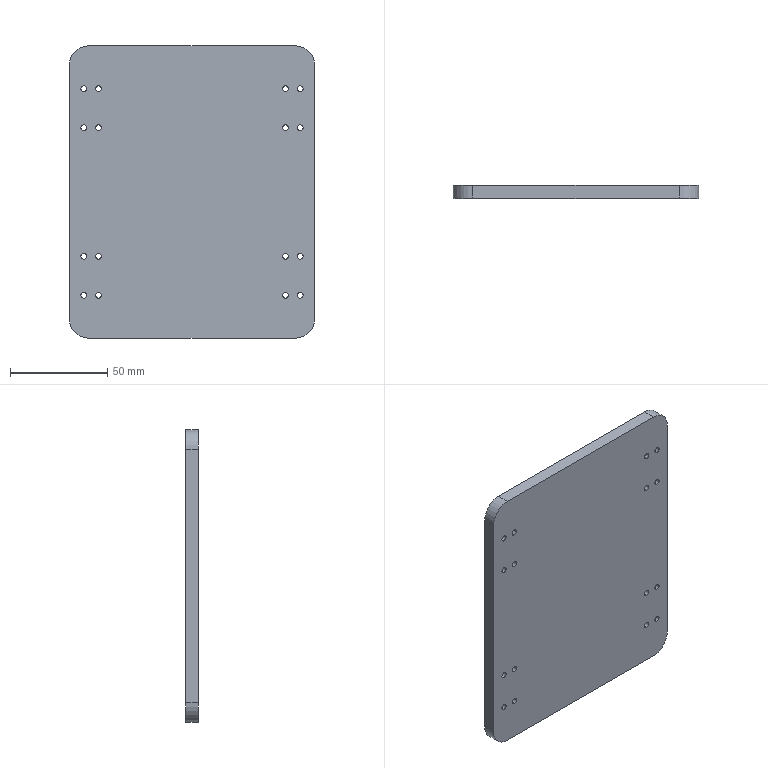Part | SolidWorks | features MirrorPattern 2, Extrusion 1, Fillet 1, ICE 1 | 1 solid | 42 faces | box 126 x 6.5 x 150 mm | volume 121557 mm3 | cylinder 36 | plane 6 | commonest cylinder face diameters 3 x32 20 x4
STEP:
#1=CARTESIAN_POINT('',(55.5,0.,54.5));
#2=VERTEX_POINT('',#1);
#3=CARTESIAN_POINT('',(55.5,0.,51.5));
#4=VERTEX_POINT('',#3);
#5=CARTESIAN_POINT('',(55.5,0.,53.));
#6=DIRECTION('',(0.,-1.,0.));
#7=DIRECTION('',(0.,0.,-1.));
#8=AXIS2_PLACEMENT_3D('',#5,#6,#7);
#9=CIRCLE('',#8,1.5);
#10=EDGE_CURVE('',#2,#4,#9,.T.);
#11=ORIENTED_EDGE('',*,*,#10,.T.);
#12=CARTESIAN_POINT('',(55.5,6.5,51.5));
#13=VERTEX_POINT('',#12);
#14=CARTESIAN_POINT('',(55.5,-3.5,51.5));
#15=DIRECTION('',(0.,1.,0.));
#16=VECTOR('',#15,1000.);
#17=LINE('',#14,#16);
#18=EDGE_CURVE('',#4,#13,#17,.T.);
#19=ORIENTED_EDGE('',*,*,#18,.T.);
#20=CARTESIAN_POINT('',(55.5,6.5,54.5));
#21=VERTEX_POINT('',#20);
#22=CARTESIAN_POINT('',(55.5,6.5,53.));
#23=DIRECTION('',(0.,1.,0.));
#24=DIRECTION('',(0.,0.,1.));
#25=AXIS2_PLACEMENT_3D('',#22,#23,#24);
#26=CIRCLE('',#25,1.5);
#27=EDGE_CURVE('',#13,#21,#26,.T.);
#28=ORIENTED_EDGE('',*,*,#27,.T.);
#29=CARTESIAN_POINT('',(55.5,-3.5,54.5));
#30=DIRECTION('',(0.,1.,0.));
#31=VECTOR('',#30,1000.);
#32=LINE('',#29,#31);
#33=EDGE_CURVE('',#2,#21,#32,.T.);
#34=ORIENTED_EDGE('',*,*,#33,.F.);
#35=EDGE_LOOP('',(#11,#19,#28,#34));
#36=FACE_OUTER_BOUND('',#35,.T.);
#37=CARTESIAN_POINT('',(55.5,-3.5,53.));
#38=DIRECTION('',(0.,1.,0.));
#39=DIRECTION('',(0.,0.,1.));
#40=AXIS2_PLACEMENT_3D('',#37,#38,#39);
#41=CYLINDRICAL_SURFACE('',#40,1.5);
#42=ADVANCED_FACE('',(#36),#41,.F.);
#43=CARTESIAN_POINT('',(48.,0.,54.5));
#44=VERTEX_POINT('',#43);
#45=CARTESIAN_POINT('',(48.,0.,51.5));
#46=VERTEX_POINT('',#45);
#47=CARTESIAN_POINT('',(48.,0.,53.));
#48=DIRECTION('',(0.,-1.,0.));
#49=DIRECTION('',(0.,0.,-1.));
#50=AXIS2_PLACEMENT_3D('',#47,#48,#49);
#51=CIRCLE('',#50,1.5);
#52=EDGE_CURVE('',#44,#46,#51,.T.);
#53=ORIENTED_EDGE('',*,*,#52,.T.);
#54=CARTESIAN_POINT('',(48.,6.5,51.5));
#55=VERTEX_POINT('',#54);
#56=CARTESIAN_POINT('',(48.,-3.5,51.5));
#57=DIRECTION('',(0.,1.,0.));
#58=VECTOR('',#57,1000.);
#59=LINE('',#56,#58);
#60=EDGE_CURVE('',#46,#55,#59,.T.);
#61=ORIENTED_EDGE('',*,*,#60,.T.);
#62=CARTESIAN_POINT('',(48.,6.5,54.5));
#63=VERTEX_POINT('',#62);
#64=CARTESIAN_POINT('',(48.,6.5,53.));
#65=DIRECTION('',(0.,1.,0.));
#66=DIRECTION('',(0.,0.,-1.));
#67=AXIS2_PLACEMENT_3D('',#64,#65,#66);
#68=CIRCLE('',#67,1.5);
#69=EDGE_CURVE('',#55,#63,#68,.T.);
#70=ORIENTED_EDGE('',*,*,#69,.T.);
#71=CARTESIAN_POINT('',(48.,-3.5,54.5));
#72=DIRECTION('',(0.,1.,0.));
#73=VECTOR('',#72,1000.);
#74=LINE('',#71,#73);
#75=EDGE_CURVE('',#44,#63,#74,.T.);
#76=ORIENTED_EDGE('',*,*,#75,.F.);
#77=EDGE_LOOP('',(#53,#61,#70,#76));
#78=FACE_OUTER_BOUND('',#77,.T.);
#79=CARTESIAN_POINT('',(48.,-3.5,53.));
#80=DIRECTION('',(0.,1.,0.));
#81=DIRECTION('',(0.,0.,1.));
#82=AXIS2_PLACEMENT_3D('',#79,#80,#81);
#83=CYLINDRICAL_SURFACE('',#82,1.5);
#84=ADVANCED_FACE('',(#78),#83,.F.);
#85=CARTESIAN_POINT('',(48.,0.,34.5));
#86=VERTEX_POINT('',#85);
#87=CARTESIAN_POINT('',(48.,0.,31.5));
#88=VERTEX_POINT('',#87);
#89=CARTESIAN_POINT('',(48.,0.,33.));
#90=DIRECTION('',(0.,-1.,0.));
#91=DIRECTION('',(0.,0.,-1.));
#92=AXIS2_PLACEMENT_3D('',#89,#90,#91);
#93=CIRCLE('',#92,1.5);
#94=EDGE_CURVE('',#86,#88,#93,.T.);
#95=ORIENTED_EDGE('',*,*,#94,.T.);
#96=CARTESIAN_POINT('',(48.,6.5,31.5));
#97=VERTEX_POINT('',#96);
#98=CARTESIAN_POINT('',(48.,-3.5,31.5));
#99=DIRECTION('',(0.,1.,0.));
#100=VECTOR('',#99,1000.);
#101=LINE('',#98,#100);
#102=EDGE_CURVE('',#88,#97,#101,.T.);
#103=ORIENTED_EDGE('',*,*,#102,.T.);
#104=CARTESIAN_POINT('',(48.,6.5,34.5));
#105=VERTEX_POINT('',#104);
#106=CARTESIAN_POINT('',(48.,6.5,33.));
#107=DIRECTION('',(0.,1.,0.));
#108=DIRECTION('',(0.,0.,1.));
#109=AXIS2_PLACEMENT_3D('',#106,#107,#108);
#110=CIRCLE('',#109,1.5);
#111=EDGE_CURVE('',#97,#105,#110,.T.);
#112=ORIENTED_EDGE('',*,*,#111,.T.);
#113=CARTESIAN_POINT('',(48.,-3.5,34.5));
#114=DIRECTION('',(0.,1.,0.));
#115=VECTOR('',#114,1000.);
#116=LINE('',#113,#115);
#117=EDGE_CURVE('',#86,#105,#116,.T.);
#118=ORIENTED_EDGE('',*,*,#117,.F.);
#119=EDGE_LOOP('',(#95,#103,#112,#118));
#120=FACE_OUTER_BOUND('',#119,.T.);
#121=CARTESIAN_POINT('',(48.,-3.5,33.));
#122=DIRECTION('',(0.,1.,0.));
#123=DIRECTION('',(0.,0.,1.));
#124=AXIS2_PLACEMENT_3D('',#121,#122,#123);
#125=CYLINDRICAL_SURFACE('',#124,1.5);
#126=ADVANCED_FACE('',(#120),#125,.F.);
#127=CARTESIAN_POINT('',(55.5,0.,34.5));
#128=VERTEX_POINT('',#127);
#129=CARTESIAN_POINT('',(55.5,0.,31.5));
#130=VERTEX_POINT('',#129);
#131=CARTESIAN_POINT('',(55.5,0.,33.));
#132=DIRECTION('',(0.,-1.,0.));
#133=DIRECTION('',(0.,0.,-1.));
#134=AXIS2_PLACEMENT_3D('',#131,#132,#133);
#135=CIRCLE('',#134,1.5);
#136=EDGE_CURVE('',#128,#130,#135,.T.);
#137=ORIENTED_EDGE('',*,*,#136,.T.);
#138=CARTESIAN_POINT('',(55.5,6.5,31.5));
#139=VERTEX_POINT('',#138);
#140=CARTESIAN_POINT('',(55.5,-3.5,31.5));
#141=DIRECTION('',(0.,1.,0.));
#142=VECTOR('',#141,1000.);
#143=LINE('',#140,#142);
#144=EDGE_CURVE('',#130,#139,#143,.T.);
#145=ORIENTED_EDGE('',*,*,#144,.T.);
#146=CARTESIAN_POINT('',(55.5,6.5,34.5));
#147=VERTEX_POINT('',#146);
#148=CARTESIAN_POINT('',(55.5,6.5,33.));
#149=DIRECTION('',(0.,1.,0.));
#150=DIRECTION('',(0.,0.,-1.));
#151=AXIS2_PLACEMENT_3D('',#148,#149,#150);
#152=CIRCLE('',#151,1.5);
#153=EDGE_CURVE('',#139,#147,#152,.T.);
#154=ORIENTED_EDGE('',*,*,#153,.T.);
#155=CARTESIAN_POINT('',(55.5,-3.5,34.5));
#156=DIRECTION('',(0.,1.,0.));
#157=VECTOR('',#156,1000.);
#158=LINE('',#155,#157);
#159=EDGE_CURVE('',#128,#147,#158,.T.);
#160=ORIENTED_EDGE('',*,*,#159,.F.);
#161=EDGE_LOOP('',(#137,#145,#154,#160));
#162=FACE_OUTER_BOUND('',#161,.T.);
#163=CARTESIAN_POINT('',(55.5,-3.5,33.));
#164=DIRECTION('',(0.,1.,0.));
#165=DIRECTION('',(0.,0.,1.));
#166=AXIS2_PLACEMENT_3D('',#163,#164,#165);
#167=CYLINDRICAL_SURFACE('',#166,1.5);
#168=ADVANCED_FACE('',(#162),#167,.F.);
#169=CARTESIAN_POINT('',(-55.5,0.,51.5));
#170=VERTEX_POINT('',#169);
#171=CARTESIAN_POINT('',(-55.5,0.,54.5));
#172=VERTEX_POINT('',#171);
#173=CARTESIAN_POINT('',(-55.5,0.,53.));
#174=DIRECTION('',(0.,1.,0.));
#175=DIRECTION('',(0.,0.,-1.));
#176=AXIS2_PLACEMENT_3D('',#173,#174,#175);
#177=CIRCLE('',#176,1.5);
#178=EDGE_CURVE('',#170,#172,#177,.T.);
#179=ORIENTED_EDGE('',*,*,#178,.F.);
#180=CARTESIAN_POINT('',(-55.5,6.5,51.5));
#181=VERTEX_POINT('',#180);
#182=CARTESIAN_POINT('',(-55.5,-3.5,51.5));
#183=DIRECTION('',(0.,1.,0.));
#184=VECTOR('',#183,1000.);
#185=LINE('',#182,#184);
#186=EDGE_CURVE('',#170,#181,#185,.T.);
#187=ORIENTED_EDGE('',*,*,#186,.T.);
#188=CARTESIAN_POINT('',(-55.5,6.5,54.5));
#189=VERTEX_POINT('',#188);
#190=CARTESIAN_POINT('',(-55.5,6.5,53.));
#191=DIRECTION('',(0.,-1.,0.));
#192=DIRECTION('',(0.,0.,1.));
#193=AXIS2_PLACEMENT_3D('',#190,#191,#192);
#194=CIRCLE('',#193,1.5);
#195=EDGE_CURVE('',#189,#181,#194,.T.);
#196=ORIENTED_EDGE('',*,*,#195,.F.);
#197=CARTESIAN_POINT('',(-55.5,-3.5,54.5));
#198=DIRECTION('',(0.,1.,0.));
#199=VECTOR('',#198,1000.);
#200=LINE('',#197,#199);
#201=EDGE_CURVE('',#172,#189,#200,.T.);
#202=ORIENTED_EDGE('',*,*,#201,.F.);
#203=EDGE_LOOP('',(#179,#187,#196,#202));
#204=FACE_OUTER_BOUND('',#203,.T.);
#205=CARTESIAN_POINT('',(-55.5,-3.5,53.));
#206=DIRECTION('',(0.,1.,0.));
#207=DIRECTION('',(0.,0.,1.));
#208=AXIS2_PLACEMENT_3D('',#205,#206,#207);
#209=CYLINDRICAL_SURFACE('',#208,1.5);
#210=ADVANCED_FACE('',(#204),#209,.F.);
#211=CARTESIAN_POINT('',(-48.,0.,51.5));
#212=VERTEX_POINT('',#211);
#213=CARTESIAN_POINT('',(-48.,0.,54.5));
#214=VERTEX_POINT('',#213);
#215=CARTESIAN_POINT('',(-48.,0.,53.));
#216=DIRECTION('',(0.,1.,0.));
#217=DIRECTION('',(0.,0.,-1.));
#218=AXIS2_PLACEMENT_3D('',#215,#216,#217);
#219=CIRCLE('',#218,1.5);
#220=EDGE_CURVE('',#212,#214,#219,.T.);
#221=ORIENTED_EDGE('',*,*,#220,.F.);
#222=CARTESIAN_POINT('',(-48.,6.5,51.5));
#223=VERTEX_POINT('',#222);
#224=CARTESIAN_POINT('',(-48.,-3.5,51.5));
#225=DIRECTION('',(0.,1.,0.));
#226=VECTOR('',#225,1000.);
#227=LINE('',#224,#226);
#228=EDGE_CURVE('',#212,#223,#227,.T.);
#229=ORIENTED_EDGE('',*,*,#228,.T.);
#230=CARTESIAN_POINT('',(-48.,6.5,54.5));
#231=VERTEX_POINT('',#230);
#232=CARTESIAN_POINT('',(-48.,6.5,53.));
#233=DIRECTION('',(0.,-1.,0.));
#234=DIRECTION('',(0.,0.,-1.));
#235=AXIS2_PLACEMENT_3D('',#232,#233,#234);
#236=CIRCLE('',#235,1.5);
#237=EDGE_CURVE('',#231,#223,#236,.T.);
#238=ORIENTED_EDGE('',*,*,#237,.F.);
#239=CARTESIAN_POINT('',(-48.,-3.5,54.5));
#240=DIRECTION('',(0.,1.,0.));
#241=VECTOR('',#240,1000.);
#242=LINE('',#239,#241);
#243=EDGE_CURVE('',#214,#231,#242,.T.);
#244=ORIENTED_EDGE('',*,*,#243,.F.);
#245=EDGE_LOOP('',(#221,#229,#238,#244));
#246=FACE_OUTER_BOUND('',#245,.T.);
#247=CARTESIAN_POINT('',(-48.,-3.5,53.));
#248=DIRECTION('',(0.,1.,0.));
#249=DIRECTION('',(0.,0.,1.));
#250=AXIS2_PLACEMENT_3D('',#247,#248,#249);
#251=CYLINDRICAL_SURFACE('',#250,1.5);
#252=ADVANCED_FACE('',(#246),#251,.F.);
#253=CARTESIAN_POINT('',(-48.,0.,31.5));
#254=VERTEX_POINT('',#253);
#255=CARTESIAN_POINT('',(-48.,0.,34.5));
#256=VERTEX_POINT('',#255);
#257=CARTESIAN_POINT('',(-48.,0.,33.));
#258=DIRECTION('',(0.,1.,0.));
#259=DIRECTION('',(0.,0.,-1.));
#260=AXIS2_PLACEMENT_3D('',#257,#258,#259);
#261=CIRCLE('',#260,1.5);
#262=EDGE_CURVE('',#254,#256,#261,.T.);
#263=ORIENTED_EDGE('',*,*,#262,.F.);
#264=CARTESIAN_POINT('',(-48.,6.5,31.5));
#265=VERTEX_POINT('',#264);
#266=CARTESIAN_POINT('',(-48.,-3.5,31.5));
#267=DIRECTION('',(0.,1.,0.));
#268=VECTOR('',#267,1000.);
#269=LINE('',#266,#268);
#270=EDGE_CURVE('',#254,#265,#269,.T.);
#271=ORIENTED_EDGE('',*,*,#270,.T.);
#272=CARTESIAN_POINT('',(-48.,6.5,34.5));
#273=VERTEX_POINT('',#272);
#274=CARTESIAN_POINT('',(-48.,6.5,33.));
#275=DIRECTION('',(0.,-1.,0.));
#276=DIRECTION('',(0.,0.,1.));
#277=AXIS2_PLACEMENT_3D('',#274,#275,#276);
#278=CIRCLE('',#277,1.5);
#279=EDGE_CURVE('',#273,#265,#278,.T.);
#280=ORIENTED_EDGE('',*,*,#279,.F.);
#281=CARTESIAN_POINT('',(-48.,-3.5,34.5));
#282=DIRECTION('',(0.,1.,0.));
#283=VECTOR('',#282,1000.);
#284=LINE('',#281,#283);
#285=EDGE_CURVE('',#256,#273,#284,.T.);
#286=ORIENTED_EDGE('',*,*,#285,.F.);
#287=EDGE_LOOP('',(#263,#271,#280,#286));
#288=FACE_OUTER_BOUND('',#287,.T.);
#289=CARTESIAN_POINT('',(-48.,-3.5,33.));
#290=DIRECTION('',(0.,1.,0.));
#291=DIRECTION('',(0.,0.,1.));
#292=AXIS2_PLACEMENT_3D('',#289,#290,#291);
#293=CYLINDRICAL_SURFACE('',#292,1.5);
#294=ADVANCED_FACE('',(#288),#293,.F.);
#295=CARTESIAN_POINT('',(-55.5,0.,31.5));
#296=VERTEX_POINT('',#295);
#297=CARTESIAN_POINT('',(-55.5,0.,34.5));
#298=VERTEX_POINT('',#297);
#299=CARTESIAN_POINT('',(-55.5,0.,33.));
#300=DIRECTION('',(0.,1.,0.));
#301=DIRECTION('',(0.,0.,-1.));
#302=AXIS2_PLACEMENT_3D('',#299,#300,#301);
#303=CIRCLE('',#302,1.5);
#304=EDGE_CURVE('',#296,#298,#303,.T.);
#305=ORIENTED_EDGE('',*,*,#304,.F.);
#306=CARTESIAN_POINT('',(-55.5,6.5,31.5));
#307=VERTEX_POINT('',#306);
#308=CARTESIAN_POINT('',(-55.5,-3.5,31.5));
#309=DIRECTION('',(0.,1.,0.));
#310=VECTOR('',#309,1000.);
#311=LINE('',#308,#310);
#312=EDGE_CURVE('',#296,#307,#311,.T.);
#313=ORIENTED_EDGE('',*,*,#312,.T.);
#314=CARTESIAN_POINT('',(-55.5,6.5,34.5));
#315=VERTEX_POINT('',#314);
#316=CARTESIAN_POINT('',(-55.5,6.5,33.));
#317=DIRECTION('',(0.,-1.,0.));
#318=DIRECTION('',(0.,0.,-1.));
#319=AXIS2_PLACEMENT_3D('',#316,#317,#318);
#320=CIRCLE('',#319,1.5);
#321=EDGE_CURVE('',#315,#307,#320,.T.);
#322=ORIENTED_EDGE('',*,*,#321,.F.);
#323=CARTESIAN_POINT('',(-55.5,-3.5,34.5));
#324=DIRECTION('',(0.,1.,0.));
#325=VECTOR('',#324,1000.);
#326=LINE('',#323,#325);
#327=EDGE_CURVE('',#298,#315,#326,.T.);
#328=ORIENTED_EDGE('',*,*,#327,.F.);
#329=EDGE_LOOP('',(#305,#313,#322,#328));
#330=FACE_OUTER_BOUND('',#329,.T.);
#331=CARTESIAN_POINT('',(-55.5,-3.5,33.));
#332=DIRECTION('',(0.,1.,0.));
#333=DIRECTION('',(0.,0.,1.));
#334=AXIS2_PLACEMENT_3D('',#331,#332,#333);
#335=CYLINDRICAL_SURFACE('',#334,1.5);
#336=ADVANCED_FACE('',(#330),#335,.F.);
#337=CARTESIAN_POINT('',(55.5,0.,-54.5));
#338=VERTEX_POINT('',#337);
#339=CARTESIAN_POINT('',(55.5,0.,-51.5));
#340=VERTEX_POINT('',#339);
#341=CARTESIAN_POINT('',(55.5,0.,-53.));
#342=DIRECTION('',(0.,1.,0.));
#343=DIRECTION('',(0.,0.,-1.));
#344=AXIS2_PLACEMENT_3D('',#341,#342,#343);
#345=CIRCLE('',#344,1.5);
#346=EDGE_CURVE('',#338,#340,#345,.T.);
#347=ORIENTED_EDGE('',*,*,#346,.F.);
#348=CARTESIAN_POINT('',(55.5,6.5,-54.5));
#349=VERTEX_POINT('',#348);
#350=CARTESIAN_POINT('',(55.5,-3.5,-54.5));
#351=DIRECTION('',(0.,1.,0.));
#352=VECTOR('',#351,1000.);
#353=LINE('',#350,#352);
#354=EDGE_CURVE('',#338,#349,#353,.T.);
#355=ORIENTED_EDGE('',*,*,#354,.T.);
#356=CARTESIAN_POINT('',(55.5,6.5,-51.5));
#357=VERTEX_POINT('',#356);
#358=CARTESIAN_POINT('',(55.5,6.5,-53.));
#359=DIRECTION('',(0.,-1.,0.));
#360=DIRECTION('',(0.,0.,-1.));
#361=AXIS2_PLACEMENT_3D('',#358,#359,#360);
#362=CIRCLE('',#361,1.5);
#363=EDGE_CURVE('',#357,#349,#362,.T.);
#364=ORIENTED_EDGE('',*,*,#363,.F.);
#365=CARTESIAN_POINT('',(55.5,-3.5,-51.5));
#366=DIRECTION('',(0.,1.,0.));
#367=VECTOR('',#366,1000.);
#368=LINE('',#365,#367);
#369=EDGE_CURVE('',#340,#357,#368,.T.);
#370=ORIENTED_EDGE('',*,*,#369,.F.);
#371=EDGE_LOOP('',(#347,#355,#364,#370));
#372=FACE_OUTER_BOUND('',#371,.T.);
#373=CARTESIAN_POINT('',(55.5,-3.5,-53.));
#374=DIRECTION('',(0.,1.,0.));
#375=DIRECTION('',(0.,0.,1.));
#376=AXIS2_PLACEMENT_3D('',#373,#374,#375);
#377=CYLINDRICAL_SURFACE('',#376,1.5);
#378=ADVANCED_FACE('',(#372),#377,.F.);
#379=CARTESIAN_POINT('',(48.,0.,-54.5));
#380=VERTEX_POINT('',#379);
#381=CARTESIAN_POINT('',(48.,0.,-51.5));
#382=VERTEX_POINT('',#381);
#383=CARTESIAN_POINT('',(48.,0.,-53.));
#384=DIRECTION('',(0.,1.,0.));
#385=DIRECTION('',(0.,0.,-1.));
#386=AXIS2_PLACEMENT_3D('',#383,#384,#385);
#387=CIRCLE('',#386,1.5);
#388=EDGE_CURVE('',#380,#382,#387,.T.);
#389=ORIENTED_EDGE('',*,*,#388,.F.);
#390=CARTESIAN_POINT('',(48.,6.5,-54.5));
#391=VERTEX_POINT('',#390);
#392=CARTESIAN_POINT('',(48.,-3.5,-54.5));
#393=DIRECTION('',(0.,1.,0.));
#394=VECTOR('',#393,1000.);
#395=LINE('',#392,#394);
#396=EDGE_CURVE('',#380,#391,#395,.T.);
#397=ORIENTED_EDGE('',*,*,#396,.T.);
#398=CARTESIAN_POINT('',(48.,6.5,-51.5));
#399=VERTEX_POINT('',#398);
#400=CARTESIAN_POINT('',(48.,6.5,-53.));
#401=DIRECTION('',(0.,-1.,0.));
#402=DIRECTION('',(0.,0.,1.));
#403=AXIS2_PLACEMENT_3D('',#400,#401,#402);
#404=CIRCLE('',#403,1.5);
#405=EDGE_CURVE('',#399,#391,#404,.T.);
#406=ORIENTED_EDGE('',*,*,#405,.F.);
#407=CARTESIAN_POINT('',(48.,-3.5,-51.5));
#408=DIRECTION('',(0.,1.,0.));
#409=VECTOR('',#408,1000.);
#410=LINE('',#407,#409);
#411=EDGE_CURVE('',#382,#399,#410,.T.);
#412=ORIENTED_EDGE('',*,*,#411,.F.);
#413=EDGE_LOOP('',(#389,#397,#406,#412));
#414=FACE_OUTER_BOUND('',#413,.T.);
#415=CARTESIAN_POINT('',(48.,-3.5,-53.));
#416=DIRECTION('',(0.,1.,0.));
#417=DIRECTION('',(0.,0.,1.));
#418=AXIS2_PLACEMENT_3D('',#415,#416,#417);
#419=CYLINDRICAL_SURFACE('',#418,1.5);
#420=ADVANCED_FACE('',(#414),#419,.F.);
#421=CARTESIAN_POINT('',(48.,0.,-34.5));
#422=VERTEX_POINT('',#421);
#423=CARTESIAN_POINT('',(48.,0.,-31.5));
#424=VERTEX_POINT('',#423);
#425=CARTESIAN_POINT('',(48.,0.,-33.));
#426=DIRECTION('',(0.,1.,0.));
#427=DIRECTION('',(0.,0.,-1.));
#428=AXIS2_PLACEMENT_3D('',#425,#426,#427);
#429=CIRCLE('',#428,1.5);
#430=EDGE_CURVE('',#422,#424,#429,.T.);
#431=ORIENTED_EDGE('',*,*,#430,.F.);
#432=CARTESIAN_POINT('',(48.,6.5,-34.5));
#433=VERTEX_POINT('',#432);
#434=CARTESIAN_POINT('',(48.,-3.5,-34.5));
#435=DIRECTION('',(0.,1.,0.));
#436=VECTOR('',#435,1000.);
#437=LINE('',#434,#436);
#438=EDGE_CURVE('',#422,#433,#437,.T.);
#439=ORIENTED_EDGE('',*,*,#438,.T.);
#440=CARTESIAN_POINT('',(48.,6.5,-31.5));
#441=VERTEX_POINT('',#440);
#442=CARTESIAN_POINT('',(48.,6.5,-33.));
#443=DIRECTION('',(0.,-1.,0.));
#444=DIRECTION('',(0.,0.,-1.));
#445=AXIS2_PLACEMENT_3D('',#442,#443,#444);
#446=CIRCLE('',#445,1.5);
#447=EDGE_CURVE('',#441,#433,#446,.T.);
#448=ORIENTED_EDGE('',*,*,#447,.F.);
#449=CARTESIAN_POINT('',(48.,-3.5,-31.5));
#450=DIRECTION('',(0.,1.,0.));
#451=VECTOR('',#450,1000.);
#452=LINE('',#449,#451);
#453=EDGE_CURVE('',#424,#441,#452,.T.);
#454=ORIENTED_EDGE('',*,*,#453,.F.);
#455=EDGE_LOOP('',(#431,#439,#448,#454));
#456=FACE_OUTER_BOUND('',#455,.T.);
#457=CARTESIAN_POINT('',(48.,-3.5,-33.));
#458=DIRECTION('',(0.,1.,0.));
#459=DIRECTION('',(0.,0.,1.));
#460=AXIS2_PLACEMENT_3D('',#457,#458,#459);
#461=CYLINDRICAL_SURFACE('',#460,1.5);
#462=ADVANCED_FACE('',(#456),#461,.F.);
#463=CARTESIAN_POINT('',(55.5,0.,-34.5));
#464=VERTEX_POINT('',#463);
#465=CARTESIAN_POINT('',(55.5,0.,-31.5));
#466=VERTEX_POINT('',#465);
#467=CARTESIAN_POINT('',(55.5,0.,-33.));
#468=DIRECTION('',(0.,1.,0.));
#469=DIRECTION('',(0.,0.,-1.));
#470=AXIS2_PLACEMENT_3D('',#467,#468,#469);
#471=CIRCLE('',#470,1.5);
#472=EDGE_CURVE('',#464,#466,#471,.T.);
#473=ORIENTED_EDGE('',*,*,#472,.F.);
#474=CARTESIAN_POINT('',(55.5,6.5,-34.5));
#475=VERTEX_POINT('',#474);
#476=CARTESIAN_POINT('',(55.5,-3.5,-34.5));
#477=DIRECTION('',(0.,1.,0.));
#478=VECTOR('',#477,1000.);
#479=LINE('',#476,#478);
#480=EDGE_CURVE('',#464,#475,#479,.T.);
#481=ORIENTED_EDGE('',*,*,#480,.T.);
#482=CARTESIAN_POINT('',(55.5,6.5,-31.5));
#483=VERTEX_POINT('',#482);
#484=CARTESIAN_POINT('',(55.5,6.5,-33.));
#485=DIRECTION('',(0.,-1.,0.));
#486=DIRECTION('',(0.,0.,1.));
#487=AXIS2_PLACEMENT_3D('',#484,#485,#486);
#488=CIRCLE('',#487,1.5);
#489=EDGE_CURVE('',#483,#475,#488,.T.);
#490=ORIENTED_EDGE('',*,*,#489,.F.);
#491=CARTESIAN_POINT('',(55.5,-3.5,-31.5));
#492=DIRECTION('',(0.,1.,0.));
#493=VECTOR('',#492,1000.);
#494=LINE('',#491,#493);
#495=EDGE_CURVE('',#466,#483,#494,.T.);
#496=ORIENTED_EDGE('',*,*,#495,.F.);
#497=EDGE_LOOP('',(#473,#481,#490,#496));
#498=FACE_OUTER_BOUND('',#497,.T.);
#499=CARTESIAN_POINT('',(55.5,-3.5,-33.));
#500=DIRECTION('',(0.,1.,0.));
#501=DIRECTION('',(0.,0.,1.));
#502=AXIS2_PLACEMENT_3D('',#499,#500,#501);
#503=CYLINDRICAL_SURFACE('',#502,1.5);
#504=ADVANCED_FACE('',(#498),#503,.F.);
#505=CARTESIAN_POINT('',(-55.5,0.,-51.5));
#506=VERTEX_POINT('',#505);
#507=CARTESIAN_POINT('',(-55.5,0.,-54.5));
#508=VERTEX_POINT('',#507);
#509=CARTESIAN_POINT('',(-55.5,0.,-53.));
#510=DIRECTION('',(0.,-1.,0.));
#511=DIRECTION('',(0.,0.,-1.));
#512=AXIS2_PLACEMENT_3D('',#509,#510,#511);
#513=CIRCLE('',#512,1.5);
#514=EDGE_CURVE('',#506,#508,#513,.T.);
#515=ORIENTED_EDGE('',*,*,#514,.T.);
#516=CARTESIAN_POINT('',(-55.5,6.5,-54.5));
#517=VERTEX_POINT('',#516);
#518=CARTESIAN_POINT('',(-55.5,-3.5,-54.5));
#519=DIRECTION('',(0.,1.,0.));
#520=VECTOR('',#519,1000.);
#521=LINE('',#518,#520);
#522=EDGE_CURVE('',#508,#517,#521,.T.);
#523=ORIENTED_EDGE('',*,*,#522,.T.);
#524=CARTESIAN_POINT('',(-55.5,6.5,-51.5));
#525=VERTEX_POINT('',#524);
#526=CARTESIAN_POINT('',(-55.5,6.5,-53.));
#527=DIRECTION('',(0.,1.,0.));
#528=DIRECTION('',(0.,0.,-1.));
#529=AXIS2_PLACEMENT_3D('',#526,#527,#528);
#530=CIRCLE('',#529,1.5);
#531=EDGE_CURVE('',#517,#525,#530,.T.);
#532=ORIENTED_EDGE('',*,*,#531,.T.);
#533=CARTESIAN_POINT('',(-55.5,-3.5,-51.5));
#534=DIRECTION('',(0.,1.,0.));
#535=VECTOR('',#534,1000.);
#536=LINE('',#533,#535);
#537=EDGE_CURVE('',#506,#525,#536,.T.);
#538=ORIENTED_EDGE('',*,*,#537,.F.);
#539=EDGE_LOOP('',(#515,#523,#532,#538));
#540=FACE_OUTER_BOUND('',#539,.T.);
#541=CARTESIAN_POINT('',(-55.5,-3.5,-53.));
#542=DIRECTION('',(0.,1.,0.));
#543=DIRECTION('',(0.,0.,1.));
#544=AXIS2_PLACEMENT_3D('',#541,#542,#543);
#545=CYLINDRICAL_SURFACE('',#544,1.5);
#546=ADVANCED_FACE('',(#540),#545,.F.);
#547=CARTESIAN_POINT('',(-48.,0.,-51.5));
#548=VERTEX_POINT('',#547);
#549=CARTESIAN_POINT('',(-48.,0.,-54.5));
#550=VERTEX_POINT('',#549);
#551=CARTESIAN_POINT('',(-48.,0.,-53.));
#552=DIRECTION('',(0.,-1.,0.));
#553=DIRECTION('',(0.,0.,-1.));
#554=AXIS2_PLACEMENT_3D('',#551,#552,#553);
#555=CIRCLE('',#554,1.5);
#556=EDGE_CURVE('',#548,#550,#555,.T.);
#557=ORIENTED_EDGE('',*,*,#556,.T.);
#558=CARTESIAN_POINT('',(-48.,6.5,-54.5));
#559=VERTEX_POINT('',#558);
#560=CARTESIAN_POINT('',(-48.,-3.5,-54.5));
#561=DIRECTION('',(0.,1.,0.));
#562=VECTOR('',#561,1000.);
#563=LINE('',#560,#562);
#564=EDGE_CURVE('',#550,#559,#563,.T.);
#565=ORIENTED_EDGE('',*,*,#564,.T.);
#566=CARTESIAN_POINT('',(-48.,6.5,-51.5));
#567=VERTEX_POINT('',#566);
#568=CARTESIAN_POINT('',(-48.,6.5,-53.));
#569=DIRECTION('',(0.,1.,0.));
#570=DIRECTION('',(0.,0.,1.));
#571=AXIS2_PLACEMENT_3D('',#568,#569,#570);
#572=CIRCLE('',#571,1.5);
#573=EDGE_CURVE('',#559,#567,#572,.T.);
#574=ORIENTED_EDGE('',*,*,#573,.T.);
#575=CARTESIAN_POINT('',(-48.,-3.5,-51.5));
#576=DIRECTION('',(0.,1.,0.));
#577=VECTOR('',#576,1000.);
#578=LINE('',#575,#577);
#579=EDGE_CURVE('',#548,#567,#578,.T.);
#580=ORIENTED_EDGE('',*,*,#579,.F.);
#581=EDGE_LOOP('',(#557,#565,#574,#580));
#582=FACE_OUTER_BOUND('',#581,.T.);
#583=CARTESIAN_POINT('',(-48.,-3.5,-53.));
#584=DIRECTION('',(0.,1.,0.));
#585=DIRECTION('',(0.,0.,1.));
#586=AXIS2_PLACEMENT_3D('',#583,#584,#585);
#587=CYLINDRICAL_SURFACE('',#586,1.5);
#588=ADVANCED_FACE('',(#582),#587,.F.);
#589=CARTESIAN_POINT('',(-48.,0.,-31.5));
#590=VERTEX_POINT('',#589);
#591=CARTESIAN_POINT('',(-48.,0.,-34.5));
#592=VERTEX_POINT('',#591);
#593=CARTESIAN_POINT('',(-48.,0.,-33.));
#594=DIRECTION('',(0.,-1.,0.));
#595=DIRECTION('',(0.,0.,-1.));
#596=AXIS2_PLACEMENT_3D('',#593,#594,#595);
#597=CIRCLE('',#596,1.5);
#598=EDGE_CURVE('',#590,#592,#597,.T.);
#599=ORIENTED_EDGE('',*,*,#598,.T.);
#600=CARTESIAN_POINT('',(-48.,6.5,-34.5));
#601=VERTEX_POINT('',#600);
#602=CARTESIAN_POINT('',(-48.,-3.5,-34.5));
#603=DIRECTION('',(0.,1.,0.));
#604=VECTOR('',#603,1000.);
#605=LINE('',#602,#604);
#606=EDGE_CURVE('',#592,#601,#605,.T.);
#607=ORIENTED_EDGE('',*,*,#606,.T.);
#608=CARTESIAN_POINT('',(-48.,6.5,-31.5));
#609=VERTEX_POINT('',#608);
#610=CARTESIAN_POINT('',(-48.,6.5,-33.));
#611=DIRECTION('',(0.,1.,0.));
#612=DIRECTION('',(0.,0.,-1.));
#613=AXIS2_PLACEMENT_3D('',#610,#611,#612);
#614=CIRCLE('',#613,1.5);
#615=EDGE_CURVE('',#601,#609,#614,.T.);
#616=ORIENTED_EDGE('',*,*,#615,.T.);
#617=CARTESIAN_POINT('',(-48.,-3.5,-31.5));
#618=DIRECTION('',(0.,1.,0.));
#619=VECTOR('',#618,1000.);
#620=LINE('',#617,#619);
#621=EDGE_CURVE('',#590,#609,#620,.T.);
#622=ORIENTED_EDGE('',*,*,#621,.F.);
#623=EDGE_LOOP('',(#599,#607,#616,#622));
#624=FACE_OUTER_BOUND('',#623,.T.);
#625=CARTESIAN_POINT('',(-48.,-3.5,-33.));
#626=DIRECTION('',(0.,1.,0.));
#627=DIRECTION('',(0.,0.,1.));
#628=AXIS2_PLACEMENT_3D('',#625,#626,#627);
#629=CYLINDRICAL_SURFACE('',#628,1.5);
#630=ADVANCED_FACE('',(#624),#629,.F.);
#631=CARTESIAN_POINT('',(-55.5,0.,-31.5));
#632=VERTEX_POINT('',#631);
#633=CARTESIAN_POINT('',(-55.5,0.,-34.5));
#634=VERTEX_POINT('',#633);
#635=CARTESIAN_POINT('',(-55.5,0.,-33.));
#636=DIRECTION('',(0.,-1.,0.));
#637=DIRECTION('',(0.,0.,-1.));
#638=AXIS2_PLACEMENT_3D('',#635,#636,#637);
#639=CIRCLE('',#638,1.5);
#640=EDGE_CURVE('',#632,#634,#639,.T.);
#641=ORIENTED_EDGE('',*,*,#640,.T.);
#642=CARTESIAN_POINT('',(-55.5,6.5,-34.5));
#643=VERTEX_POINT('',#642);
#644=CARTESIAN_POINT('',(-55.5,-3.5,-34.5));
#645=DIRECTION('',(0.,1.,0.));
#646=VECTOR('',#645,1000.);
#647=LINE('',#644,#646);
#648=EDGE_CURVE('',#634,#643,#647,.T.);
#649=ORIENTED_EDGE('',*,*,#648,.T.);
#650=CARTESIAN_POINT('',(-55.5,6.5,-31.5));
#651=VERTEX_POINT('',#650);
#652=CARTESIAN_POINT('',(-55.5,6.5,-33.));
#653=DIRECTION('',(0.,1.,0.));
#654=DIRECTION('',(0.,0.,1.));
#655=AXIS2_PLACEMENT_3D('',#652,#653,#654);
#656=CIRCLE('',#655,1.5);
#657=EDGE_CURVE('',#643,#651,#656,.T.);
#658=ORIENTED_EDGE('',*,*,#657,.T.);
#659=CARTESIAN_POINT('',(-55.5,-3.5,-31.5));
#660=DIRECTION('',(0.,1.,0.));
#661=VECTOR('',#660,1000.);
#662=LINE('',#659,#661);
#663=EDGE_CURVE('',#632,#651,#662,.T.);
#664=ORIENTED_EDGE('',*,*,#663,.F.);
#665=EDGE_LOOP('',(#641,#649,#658,#664));
#666=FACE_OUTER_BOUND('',#665,.T.);
#667=CARTESIAN_POINT('',(-55.5,-3.5,-33.));
#668=DIRECTION('',(0.,1.,0.));
#669=DIRECTION('',(0.,0.,1.));
#670=AXIS2_PLACEMENT_3D('',#667,#668,#669);
#671=CYLINDRICAL_SURFACE('',#670,1.5);
#672=ADVANCED_FACE('',(#666),#671,.F.);
#673=CARTESIAN_POINT('',(63.,6.5,65.));
#674=VERTEX_POINT('',#673);
#675=CARTESIAN_POINT('',(63.,6.5,-65.));
#676=VERTEX_POINT('',#675);
#677=CARTESIAN_POINT('',(63.,6.5,75.));
#678=DIRECTION('',(0.,0.,-1.));
#679=VECTOR('',#678,1000.);
#680=LINE('',#677,#679);
#681=EDGE_CURVE('',#674,#676,#680,.T.);
#682=ORIENTED_EDGE('',*,*,#681,.F.);
#683=CARTESIAN_POINT('',(63.,0.,65.));
#684=VERTEX_POINT('',#683);
#685=CARTESIAN_POINT('',(63.,6.5,65.));
#686=DIRECTION('',(0.,-1.,0.));
#687=VECTOR('',#686,1000.);
#688=LINE('',#685,#687);
#689=EDGE_CURVE('',#674,#684,#688,.T.);
#690=ORIENTED_EDGE('',*,*,#689,.T.);
#691=CARTESIAN_POINT('',(63.,0.,-65.));
#692=VERTEX_POINT('',#691);
#693=CARTESIAN_POINT('',(63.,0.,75.));
#694=DIRECTION('',(0.,0.,-1.));
#695=VECTOR('',#694,1000.);
#696=LINE('',#693,#695);
#697=EDGE_CURVE('',#684,#692,#696,.T.);
#698=ORIENTED_EDGE('',*,*,#697,.T.);
#699=CARTESIAN_POINT('',(63.,6.5,-65.));
#700=DIRECTION('',(0.,1.,0.));
#701=VECTOR('',#700,1000.);
#702=LINE('',#699,#701);
#703=EDGE_CURVE('',#692,#676,#702,.T.);
#704=ORIENTED_EDGE('',*,*,#703,.T.);
#705=EDGE_LOOP('',(#682,#690,#698,#704));
#706=FACE_OUTER_BOUND('',#705,.T.);
#707=CARTESIAN_POINT('',(63.,6.5,75.));
#708=DIRECTION('',(-1.,0.,0.));
#709=DIRECTION('',(0.,0.,1.));
#710=AXIS2_PLACEMENT_3D('',#707,#708,#709);
#711=PLANE('',#710);
#712=ADVANCED_FACE('',(#706),#711,.F.);
#713=CARTESIAN_POINT('',(53.,6.5,-75.));
#714=VERTEX_POINT('',#713);
#715=CARTESIAN_POINT('',(-53.,6.5,-75.));
#716=VERTEX_POINT('',#715);
#717=CARTESIAN_POINT('',(-63.,6.5,-75.));
#718=DIRECTION('',(-1.,0.,0.));
#719=VECTOR('',#718,1000.);
#720=LINE('',#717,#719);
#721=EDGE_CURVE('',#714,#716,#720,.T.);
#722=ORIENTED_EDGE('',*,*,#721,.F.);
#723=CARTESIAN_POINT('',(53.,0.,-75.));
#724=VERTEX_POINT('',#723);
#725=CARTESIAN_POINT('',(53.,6.5,-75.));
#726=DIRECTION('',(0.,-1.,0.));
#727=VECTOR('',#726,1000.);
#728=LINE('',#725,#727);
#729=EDGE_CURVE('',#714,#724,#728,.T.);
#730=ORIENTED_EDGE('',*,*,#729,.T.);
#731=CARTESIAN_POINT('',(-53.,0.,-75.));
#732=VERTEX_POINT('',#731);
#733=CARTESIAN_POINT('',(-63.,0.,-75.));
#734=DIRECTION('',(-1.,0.,0.));
#735=VECTOR('',#734,1000.);
#736=LINE('',#733,#735);
#737=EDGE_CURVE('',#724,#732,#736,.T.);
#738=ORIENTED_EDGE('',*,*,#737,.T.);
#739=CARTESIAN_POINT('',(-53.,6.5,-75.));
#740=DIRECTION('',(0.,1.,0.));
#741=VECTOR('',#740,1000.);
#742=LINE('',#739,#741);
#743=EDGE_CURVE('',#732,#716,#742,.T.);
#744=ORIENTED_EDGE('',*,*,#743,.T.);
#745=EDGE_LOOP('',(#722,#730,#738,#744));
#746=FACE_OUTER_BOUND('',#745,.T.);
#747=CARTESIAN_POINT('',(-63.,6.5,-75.));
#748=DIRECTION('',(0.,0.,1.));
#749=DIRECTION('',(1.,0.,0.));
#750=AXIS2_PLACEMENT_3D('',#747,#748,#749);
#751=PLANE('',#750);
#752=ADVANCED_FACE('',(#746),#751,.F.);
#753=CARTESIAN_POINT('',(-63.,0.,-65.));
#754=VERTEX_POINT('',#753);
#755=CARTESIAN_POINT('',(-63.,0.,65.));
#756=VERTEX_POINT('',#755);
#757=CARTESIAN_POINT('',(-63.,0.,75.));
#758=DIRECTION('',(0.,0.,1.));
#759=VECTOR('',#758,1000.);
#760=LINE('',#757,#759);
#761=EDGE_CURVE('',#754,#756,#760,.T.);
#762=ORIENTED_EDGE('',*,*,#761,.T.);
#763=CARTESIAN_POINT('',(-63.,6.5,65.));
#764=VERTEX_POINT('',#763);
#765=CARTESIAN_POINT('',(-63.,6.5,65.));
#766=DIRECTION('',(0.,1.,0.));
#767=VECTOR('',#766,1000.);
#768=LINE('',#765,#767);
#769=EDGE_CURVE('',#756,#764,#768,.T.);
#770=ORIENTED_EDGE('',*,*,#769,.T.);
#771=CARTESIAN_POINT('',(-63.,6.5,-65.));
#772=VERTEX_POINT('',#771);
#773=CARTESIAN_POINT('',(-63.,6.5,75.));
#774=DIRECTION('',(0.,0.,1.));
#775=VECTOR('',#774,1000.);
#776=LINE('',#773,#775);
#777=EDGE_CURVE('',#772,#764,#776,.T.);
#778=ORIENTED_EDGE('',*,*,#777,.F.);
#779=CARTESIAN_POINT('',(-63.,6.5,-65.));
#780=DIRECTION('',(0.,-1.,0.));
#781=VECTOR('',#780,1000.);
#782=LINE('',#779,#781);
#783=EDGE_CURVE('',#772,#754,#782,.T.);
#784=ORIENTED_EDGE('',*,*,#783,.T.);
#785=EDGE_LOOP('',(#762,#770,#778,#784));
#786=FACE_OUTER_BOUND('',#785,.T.);
#787=CARTESIAN_POINT('',(-63.,6.5,75.));
#788=DIRECTION('',(1.,0.,0.));
#789=DIRECTION('',(0.,0.,-1.));
#790=AXIS2_PLACEMENT_3D('',#787,#788,#789);
#791=PLANE('',#790);
#792=ADVANCED_FACE('',(#786),#791,.F.);
#793=CARTESIAN_POINT('',(-53.,0.,75.));
#794=VERTEX_POINT('',#793);
#795=CARTESIAN_POINT('',(53.,0.,75.));
#796=VERTEX_POINT('',#795);
#797=CARTESIAN_POINT('',(-63.,0.,75.));
#798=DIRECTION('',(1.,0.,0.));
#799=VECTOR('',#798,1000.);
#800=LINE('',#797,#799);
#801=EDGE_CURVE('',#794,#796,#800,.T.);
#802=ORIENTED_EDGE('',*,*,#801,.T.);
#803=CARTESIAN_POINT('',(53.,6.5,75.));
#804=VERTEX_POINT('',#803);
#805=CARTESIAN_POINT('',(53.,6.5,75.));
#806=DIRECTION('',(0.,1.,0.));
#807=VECTOR('',#806,1000.);
#808=LINE('',#805,#807);
#809=EDGE_CURVE('',#796,#804,#808,.T.);
#810=ORIENTED_EDGE('',*,*,#809,.T.);
#811=CARTESIAN_POINT('',(-53.,6.5,75.));
#812=VERTEX_POINT('',#811);
#813=CARTESIAN_POINT('',(-63.,6.5,75.));
#814=DIRECTION('',(1.,0.,0.));
#815=VECTOR('',#814,1000.);
#816=LINE('',#813,#815);
#817=EDGE_CURVE('',#812,#804,#816,.T.);
#818=ORIENTED_EDGE('',*,*,#817,.F.);
#819=CARTESIAN_POINT('',(-53.,6.5,75.));
#820=DIRECTION('',(0.,-1.,0.));
#821=VECTOR('',#820,1000.);
#822=LINE('',#819,#821);
#823=EDGE_CURVE('',#812,#794,#822,.T.);
#824=ORIENTED_EDGE('',*,*,#823,.T.);
#825=EDGE_LOOP('',(#802,#810,#818,#824));
#826=FACE_OUTER_BOUND('',#825,.T.);
#827=CARTESIAN_POINT('',(-63.,6.5,75.));
#828=DIRECTION('',(0.,0.,-1.));
#829=DIRECTION('',(-1.,0.,0.));
#830=AXIS2_PLACEMENT_3D('',#827,#828,#829);
#831=PLANE('',#830);
#832=ADVANCED_FACE('',(#826),#831,.F.);
#833=CARTESIAN_POINT('',(55.5,6.5,53.));
#834=DIRECTION('',(0.,1.,0.));
#835=DIRECTION('',(0.,0.,1.));
#836=AXIS2_PLACEMENT_3D('',#833,#834,#835);
#837=CIRCLE('',#836,1.5);
#838=EDGE_CURVE('',#21,#13,#837,.T.);
#839=ORIENTED_EDGE('',*,*,#838,.F.);
#840=ORIENTED_EDGE('',*,*,#27,.F.);
#841=EDGE_LOOP('',(#839,#840));
#842=FACE_BOUND('',#841,.T.);
#843=CARTESIAN_POINT('',(48.,6.5,53.));
#844=DIRECTION('',(0.,1.,0.));
#845=DIRECTION('',(0.,0.,-1.));
#846=AXIS2_PLACEMENT_3D('',#843,#844,#845);
#847=CIRCLE('',#846,1.5);
#848=EDGE_CURVE('',#63,#55,#847,.T.);
#849=ORIENTED_EDGE('',*,*,#848,.F.);
#850=ORIENTED_EDGE('',*,*,#69,.F.);
#851=EDGE_LOOP('',(#849,#850));
#852=FACE_BOUND('',#851,.T.);
#853=CARTESIAN_POINT('',(48.,6.5,33.));
#854=DIRECTION('',(0.,1.,0.));
#855=DIRECTION('',(0.,0.,1.));
#856=AXIS2_PLACEMENT_3D('',#853,#854,#855);
#857=CIRCLE('',#856,1.5);
#858=EDGE_CURVE('',#105,#97,#857,.T.);
#859=ORIENTED_EDGE('',*,*,#858,.F.);
#860=ORIENTED_EDGE('',*,*,#111,.F.);
#861=EDGE_LOOP('',(#859,#860));
#862=FACE_BOUND('',#861,.T.);
#863=CARTESIAN_POINT('',(55.5,6.5,33.));
#864=DIRECTION('',(0.,1.,0.));
#865=DIRECTION('',(0.,0.,-1.));
#866=AXIS2_PLACEMENT_3D('',#863,#864,#865);
#867=CIRCLE('',#866,1.5);
#868=EDGE_CURVE('',#147,#139,#867,.T.);
#869=ORIENTED_EDGE('',*,*,#868,.F.);
#870=ORIENTED_EDGE('',*,*,#153,.F.);
#871=EDGE_LOOP('',(#869,#870));
#872=FACE_BOUND('',#871,.T.);
#873=ORIENTED_EDGE('',*,*,#195,.T.);
#874=CARTESIAN_POINT('',(-55.5,6.5,53.));
#875=DIRECTION('',(0.,-1.,0.));
#876=DIRECTION('',(0.,0.,1.));
#877=AXIS2_PLACEMENT_3D('',#874,#875,#876);
#878=CIRCLE('',#877,1.5);
#879=EDGE_CURVE('',#181,#189,#878,.T.);
#880=ORIENTED_EDGE('',*,*,#879,.T.);
#881=EDGE_LOOP('',(#873,#880));
#882=FACE_BOUND('',#881,.T.);
#883=ORIENTED_EDGE('',*,*,#237,.T.);
#884=CARTESIAN_POINT('',(-48.,6.5,53.));
#885=DIRECTION('',(0.,-1.,0.));
#886=DIRECTION('',(0.,0.,-1.));
#887=AXIS2_PLACEMENT_3D('',#884,#885,#886);
#888=CIRCLE('',#887,1.5);
#889=EDGE_CURVE('',#223,#231,#888,.T.);
#890=ORIENTED_EDGE('',*,*,#889,.T.);
#891=EDGE_LOOP('',(#883,#890));
#892=FACE_BOUND('',#891,.T.);
#893=ORIENTED_EDGE('',*,*,#279,.T.);
#894=CARTESIAN_POINT('',(-48.,6.5,33.));
#895=DIRECTION('',(0.,-1.,0.));
#896=DIRECTION('',(0.,0.,1.));
#897=AXIS2_PLACEMENT_3D('',#894,#895,#896);
#898=CIRCLE('',#897,1.5);
#899=EDGE_CURVE('',#265,#273,#898,.T.);
#900=ORIENTED_EDGE('',*,*,#899,.T.);
#901=EDGE_LOOP('',(#893,#900));
#902=FACE_BOUND('',#901,.T.);
#903=ORIENTED_EDGE('',*,*,#321,.T.);
#904=CARTESIAN_POINT('',(-55.5,6.5,33.));
#905=DIRECTION('',(0.,-1.,0.));
#906=DIRECTION('',(0.,0.,-1.));
#907=AXIS2_PLACEMENT_3D('',#904,#905,#906);
#908=CIRCLE('',#907,1.5);
#909=EDGE_CURVE('',#307,#315,#908,.T.);
#910=ORIENTED_EDGE('',*,*,#909,.T.);
#911=EDGE_LOOP('',(#903,#910));
#912=FACE_BOUND('',#911,.T.);
#913=ORIENTED_EDGE('',*,*,#363,.T.);
#914=CARTESIAN_POINT('',(55.5,6.5,-53.));
#915=DIRECTION('',(0.,-1.,0.));
#916=DIRECTION('',(0.,0.,-1.));
#917=AXIS2_PLACEMENT_3D('',#914,#915,#916);
#918=CIRCLE('',#917,1.5);
#919=EDGE_CURVE('',#349,#357,#918,.T.);
#920=ORIENTED_EDGE('',*,*,#919,.T.);
#921=EDGE_LOOP('',(#913,#920));
#922=FACE_BOUND('',#921,.T.);
#923=ORIENTED_EDGE('',*,*,#405,.T.);
#924=CARTESIAN_POINT('',(48.,6.5,-53.));
#925=DIRECTION('',(0.,-1.,0.));
#926=DIRECTION('',(0.,0.,1.));
#927=AXIS2_PLACEMENT_3D('',#924,#925,#926);
#928=CIRCLE('',#927,1.5);
#929=EDGE_CURVE('',#391,#399,#928,.T.);
#930=ORIENTED_EDGE('',*,*,#929,.T.);
#931=EDGE_LOOP('',(#923,#930));
#932=FACE_BOUND('',#931,.T.);
#933=ORIENTED_EDGE('',*,*,#447,.T.);
#934=CARTESIAN_POINT('',(48.,6.5,-33.));
#935=DIRECTION('',(0.,-1.,0.));
#936=DIRECTION('',(0.,0.,-1.));
#937=AXIS2_PLACEMENT_3D('',#934,#935,#936);
#938=CIRCLE('',#937,1.5);
#939=EDGE_CURVE('',#433,#441,#938,.T.);
#940=ORIENTED_EDGE('',*,*,#939,.T.);
#941=EDGE_LOOP('',(#933,#940));
#942=FACE_BOUND('',#941,.T.);
#943=ORIENTED_EDGE('',*,*,#489,.T.);
#944=CARTESIAN_POINT('',(55.5,6.5,-33.));
#945=DIRECTION('',(0.,-1.,0.));
#946=DIRECTION('',(0.,0.,1.));
#947=AXIS2_PLACEMENT_3D('',#944,#945,#946);
#948=CIRCLE('',#947,1.5);
#949=EDGE_CURVE('',#475,#483,#948,.T.);
#950=ORIENTED_EDGE('',*,*,#949,.T.);
#951=EDGE_LOOP('',(#943,#950));
#952=FACE_BOUND('',#951,.T.);
#953=CARTESIAN_POINT('',(-55.5,6.5,-53.));
#954=DIRECTION('',(0.,1.,0.));
#955=DIRECTION('',(0.,0.,-1.));
#956=AXIS2_PLACEMENT_3D('',#953,#954,#955);
#957=CIRCLE('',#956,1.5);
#958=EDGE_CURVE('',#525,#517,#957,.T.);
#959=ORIENTED_EDGE('',*,*,#958,.F.);
#960=ORIENTED_EDGE('',*,*,#531,.F.);
#961=EDGE_LOOP('',(#959,#960));
#962=FACE_BOUND('',#961,.T.);
#963=CARTESIAN_POINT('',(-48.,6.5,-53.));
#964=DIRECTION('',(0.,1.,0.));
#965=DIRECTION('',(0.,0.,1.));
#966=AXIS2_PLACEMENT_3D('',#963,#964,#965);
#967=CIRCLE('',#966,1.5);
#968=EDGE_CURVE('',#567,#559,#967,.T.);
#969=ORIENTED_EDGE('',*,*,#968,.F.);
#970=ORIENTED_EDGE('',*,*,#573,.F.);
#971=EDGE_LOOP('',(#969,#970));
#972=FACE_BOUND('',#971,.T.);
#973=CARTESIAN_POINT('',(-48.,6.5,-33.));
#974=DIRECTION('',(0.,1.,0.));
#975=DIRECTION('',(0.,0.,-1.));
#976=AXIS2_PLACEMENT_3D('',#973,#974,#975);
#977=CIRCLE('',#976,1.5);
#978=EDGE_CURVE('',#609,#601,#977,.T.);
#979=ORIENTED_EDGE('',*,*,#978,.F.);
#980=ORIENTED_EDGE('',*,*,#615,.F.);
#981=EDGE_LOOP('',(#979,#980));
#982=FACE_BOUND('',#981,.T.);
#983=CARTESIAN_POINT('',(-55.5,6.5,-33.));
#984=DIRECTION('',(0.,1.,0.));
#985=DIRECTION('',(0.,0.,1.));
#986=AXIS2_PLACEMENT_3D('',#983,#984,#985);
#987=CIRCLE('',#986,1.5);
#988=EDGE_CURVE('',#651,#643,#987,.T.);
#989=ORIENTED_EDGE('',*,*,#988,.F.);
#990=ORIENTED_EDGE('',*,*,#657,.F.);
#991=EDGE_LOOP('',(#989,#990));
#992=FACE_BOUND('',#991,.T.);
#993=ORIENTED_EDGE('',*,*,#817,.T.);
#994=CARTESIAN_POINT('',(53.,6.5,65.));
#995=DIRECTION('',(0.,1.,0.));
#996=DIRECTION('',(0.,0.,-1.));
#997=AXIS2_PLACEMENT_3D('',#994,#995,#996);
#998=CIRCLE('',#997,10.);
#999=EDGE_CURVE('',#804,#674,#998,.T.);
#1000=ORIENTED_EDGE('',*,*,#999,.T.);
#1001=ORIENTED_EDGE('',*,*,#681,.T.);
#1002=CARTESIAN_POINT('',(53.,6.5,-65.));
#1003=DIRECTION('',(0.,1.,0.));
#1004=DIRECTION('',(0.,0.,-1.));
#1005=AXIS2_PLACEMENT_3D('',#1002,#1003,#1004);
#1006=CIRCLE('',#1005,10.);
#1007=EDGE_CURVE('',#676,#714,#1006,.T.);
#1008=ORIENTED_EDGE('',*,*,#1007,.T.);
#1009=ORIENTED_EDGE('',*,*,#721,.T.);
#1010=CARTESIAN_POINT('',(-53.,6.5,-65.));
#1011=DIRECTION('',(0.,1.,0.));
#1012=DIRECTION('',(0.,0.,-1.));
#1013=AXIS2_PLACEMENT_3D('',#1010,#1011,#1012);
#1014=CIRCLE('',#1013,10.);
#1015=EDGE_CURVE('',#716,#772,#1014,.T.);
#1016=ORIENTED_EDGE('',*,*,#1015,.T.);
#1017=ORIENTED_EDGE('',*,*,#777,.T.);
#1018=CARTESIAN_POINT('',(-53.,6.5,65.));
#1019=DIRECTION('',(0.,1.,0.));
#1020=DIRECTION('',(0.,0.,-1.));
#1021=AXIS2_PLACEMENT_3D('',#1018,#1019,#1020);
#1022=CIRCLE('',#1021,10.);
#1023=EDGE_CURVE('',#764,#812,#1022,.T.);
#1024=ORIENTED_EDGE('',*,*,#1023,.T.);
#1025=EDGE_LOOP('',(#993,#1000,#1001,#1008,#1009,#1016,#1017,#1024));
#1026=FACE_OUTER_BOUND('',#1025,.T.);
#1027=CARTESIAN_POINT('',(0.,6.5,0.));
#1028=DIRECTION('',(0.,-1.,0.));
#1029=DIRECTION('',(0.,0.,-1.));
#1030=AXIS2_PLACEMENT_3D('',#1027,#1028,#1029);
#1031=PLANE('',#1030);
#1032=ADVANCED_FACE('',(#842,#852,#862,#872,#882,#892,#902,#912,#922,#932,#942,#952,#962,#972,#982,#992,#1026),#1031,.F.);
#1033=ORIENTED_EDGE('',*,*,#10,.F.);
#1034=CARTESIAN_POINT('',(55.5,0.,53.));
#1035=DIRECTION('',(0.,-1.,0.));
#1036=DIRECTION('',(0.,0.,-1.));
#1037=AXIS2_PLACEMENT_3D('',#1034,#1035,#1036);
#1038=CIRCLE('',#1037,1.5);
#1039=EDGE_CURVE('',#4,#2,#1038,.T.);
#1040=ORIENTED_EDGE('',*,*,#1039,.F.);
#1041=EDGE_LOOP('',(#1033,#1040));
#1042=FACE_BOUND('',#1041,.T.);
#1043=ORIENTED_EDGE('',*,*,#52,.F.);
#1044=CARTESIAN_POINT('',(48.,0.,53.));
#1045=DIRECTION('',(0.,-1.,0.));
#1046=DIRECTION('',(0.,0.,-1.));
#1047=AXIS2_PLACEMENT_3D('',#1044,#1045,#1046);
#1048=CIRCLE('',#1047,1.5);
#1049=EDGE_CURVE('',#46,#44,#1048,.T.);
#1050=ORIENTED_EDGE('',*,*,#1049,.F.);
#1051=EDGE_LOOP('',(#1043,#1050));
#1052=FACE_BOUND('',#1051,.T.);
#1053=ORIENTED_EDGE('',*,*,#94,.F.);
#1054=CARTESIAN_POINT('',(48.,0.,33.));
#1055=DIRECTION('',(0.,-1.,0.));
#1056=DIRECTION('',(0.,0.,-1.));
#1057=AXIS2_PLACEMENT_3D('',#1054,#1055,#1056);
#1058=CIRCLE('',#1057,1.5);
#1059=EDGE_CURVE('',#88,#86,#1058,.T.);
#1060=ORIENTED_EDGE('',*,*,#1059,.F.);
#1061=EDGE_LOOP('',(#1053,#1060));
#1062=FACE_BOUND('',#1061,.T.);
#1063=ORIENTED_EDGE('',*,*,#136,.F.);
#1064=CARTESIAN_POINT('',(55.5,0.,33.));
#1065=DIRECTION('',(0.,-1.,0.));
#1066=DIRECTION('',(0.,0.,-1.));
#1067=AXIS2_PLACEMENT_3D('',#1064,#1065,#1066);
#1068=CIRCLE('',#1067,1.5);
#1069=EDGE_CURVE('',#130,#128,#1068,.T.);
#1070=ORIENTED_EDGE('',*,*,#1069,.F.);
#1071=EDGE_LOOP('',(#1063,#1070));
#1072=FACE_BOUND('',#1071,.T.);
#1073=CARTESIAN_POINT('',(-55.5,0.,53.));
#1074=DIRECTION('',(0.,1.,0.));
#1075=DIRECTION('',(0.,0.,-1.));
#1076=AXIS2_PLACEMENT_3D('',#1073,#1074,#1075);
#1077=CIRCLE('',#1076,1.5);
#1078=EDGE_CURVE('',#172,#170,#1077,.T.);
#1079=ORIENTED_EDGE('',*,*,#1078,.T.);
#1080=ORIENTED_EDGE('',*,*,#178,.T.);
#1081=EDGE_LOOP('',(#1079,#1080));
#1082=FACE_BOUND('',#1081,.T.);
#1083=CARTESIAN_POINT('',(-48.,0.,53.));
#1084=DIRECTION('',(0.,1.,0.));
#1085=DIRECTION('',(0.,0.,-1.));
#1086=AXIS2_PLACEMENT_3D('',#1083,#1084,#1085);
#1087=CIRCLE('',#1086,1.5);
#1088=EDGE_CURVE('',#214,#212,#1087,.T.);
#1089=ORIENTED_EDGE('',*,*,#1088,.T.);
#1090=ORIENTED_EDGE('',*,*,#220,.T.);
#1091=EDGE_LOOP('',(#1089,#1090));
#1092=FACE_BOUND('',#1091,.T.);
#1093=CARTESIAN_POINT('',(-48.,0.,33.));
#1094=DIRECTION('',(0.,1.,0.));
#1095=DIRECTION('',(0.,0.,-1.));
#1096=AXIS2_PLACEMENT_3D('',#1093,#1094,#1095);
#1097=CIRCLE('',#1096,1.5);
#1098=EDGE_CURVE('',#256,#254,#1097,.T.);
#1099=ORIENTED_EDGE('',*,*,#1098,.T.);
#1100=ORIENTED_EDGE('',*,*,#262,.T.);
#1101=EDGE_LOOP('',(#1099,#1100));
#1102=FACE_BOUND('',#1101,.T.);
#1103=CARTESIAN_POINT('',(-55.5,0.,33.));
#1104=DIRECTION('',(0.,1.,0.));
#1105=DIRECTION('',(0.,0.,-1.));
#1106=AXIS2_PLACEMENT_3D('',#1103,#1104,#1105);
#1107=CIRCLE('',#1106,1.5);
#1108=EDGE_CURVE('',#298,#296,#1107,.T.);
#1109=ORIENTED_EDGE('',*,*,#1108,.T.);
#1110=ORIENTED_EDGE('',*,*,#304,.T.);
#1111=EDGE_LOOP('',(#1109,#1110));
#1112=FACE_BOUND('',#1111,.T.);
#1113=CARTESIAN_POINT('',(55.5,0.,-53.));
#1114=DIRECTION('',(0.,1.,0.));
#1115=DIRECTION('',(0.,0.,-1.));
#1116=AXIS2_PLACEMENT_3D('',#1113,#1114,#1115);
#1117=CIRCLE('',#1116,1.5);
#1118=EDGE_CURVE('',#340,#338,#1117,.T.);
#1119=ORIENTED_EDGE('',*,*,#1118,.T.);
#1120=ORIENTED_EDGE('',*,*,#346,.T.);
#1121=EDGE_LOOP('',(#1119,#1120));
#1122=FACE_BOUND('',#1121,.T.);
#1123=CARTESIAN_POINT('',(48.,0.,-53.));
#1124=DIRECTION('',(0.,1.,0.));
#1125=DIRECTION('',(0.,0.,-1.));
#1126=AXIS2_PLACEMENT_3D('',#1123,#1124,#1125);
#1127=CIRCLE('',#1126,1.5);
#1128=EDGE_CURVE('',#382,#380,#1127,.T.);
#1129=ORIENTED_EDGE('',*,*,#1128,.T.);
#1130=ORIENTED_EDGE('',*,*,#388,.T.);
#1131=EDGE_LOOP('',(#1129,#1130));
#1132=FACE_BOUND('',#1131,.T.);
#1133=CARTESIAN_POINT('',(48.,0.,-33.));
#1134=DIRECTION('',(0.,1.,0.));
#1135=DIRECTION('',(0.,0.,-1.));
#1136=AXIS2_PLACEMENT_3D('',#1133,#1134,#1135);
#1137=CIRCLE('',#1136,1.5);
#1138=EDGE_CURVE('',#424,#422,#1137,.T.);
#1139=ORIENTED_EDGE('',*,*,#1138,.T.);
#1140=ORIENTED_EDGE('',*,*,#430,.T.);
#1141=EDGE_LOOP('',(#1139,#1140));
#1142=FACE_BOUND('',#1141,.T.);
#1143=CARTESIAN_POINT('',(55.5,0.,-33.));
#1144=DIRECTION('',(0.,1.,0.));
#1145=DIRECTION('',(0.,0.,-1.));
#1146=AXIS2_PLACEMENT_3D('',#1143,#1144,#1145);
#1147=CIRCLE('',#1146,1.5);
#1148=EDGE_CURVE('',#466,#464,#1147,.T.);
#1149=ORIENTED_EDGE('',*,*,#1148,.T.);
#1150=ORIENTED_EDGE('',*,*,#472,.T.);
#1151=EDGE_LOOP('',(#1149,#1150));
#1152=FACE_BOUND('',#1151,.T.);
#1153=ORIENTED_EDGE('',*,*,#514,.F.);
#1154=CARTESIAN_POINT('',(-55.5,0.,-53.));
#1155=DIRECTION('',(0.,-1.,0.));
#1156=DIRECTION('',(0.,0.,-1.));
#1157=AXIS2_PLACEMENT_3D('',#1154,#1155,#1156);
#1158=CIRCLE('',#1157,1.5);
#1159=EDGE_CURVE('',#508,#506,#1158,.T.);
#1160=ORIENTED_EDGE('',*,*,#1159,.F.);
#1161=EDGE_LOOP('',(#1153,#1160));
#1162=FACE_BOUND('',#1161,.T.);
#1163=ORIENTED_EDGE('',*,*,#556,.F.);
#1164=CARTESIAN_POINT('',(-48.,0.,-53.));
#1165=DIRECTION('',(0.,-1.,0.));
#1166=DIRECTION('',(0.,0.,-1.));
#1167=AXIS2_PLACEMENT_3D('',#1164,#1165,#1166);
#1168=CIRCLE('',#1167,1.5);
#1169=EDGE_CURVE('',#550,#548,#1168,.T.);
#1170=ORIENTED_EDGE('',*,*,#1169,.F.);
#1171=EDGE_LOOP('',(#1163,#1170));
#1172=FACE_BOUND('',#1171,.T.);
#1173=ORIENTED_EDGE('',*,*,#598,.F.);
#1174=CARTESIAN_POINT('',(-48.,0.,-33.));
#1175=DIRECTION('',(0.,-1.,0.));
#1176=DIRECTION('',(0.,0.,-1.));
#1177=AXIS2_PLACEMENT_3D('',#1174,#1175,#1176);
#1178=CIRCLE('',#1177,1.5);
#1179=EDGE_CURVE('',#592,#590,#1178,.T.);
#1180=ORIENTED_EDGE('',*,*,#1179,.F.);
#1181=EDGE_LOOP('',(#1173,#1180));
#1182=FACE_BOUND('',#1181,.T.);
#1183=ORIENTED_EDGE('',*,*,#640,.F.);
#1184=CARTESIAN_POINT('',(-55.5,0.,-33.));
#1185=DIRECTION('',(0.,-1.,0.));
#1186=DIRECTION('',(0.,0.,-1.));
#1187=AXIS2_PLACEMENT_3D('',#1184,#1185,#1186);
#1188=CIRCLE('',#1187,1.5);
#1189=EDGE_CURVE('',#634,#632,#1188,.T.);
#1190=ORIENTED_EDGE('',*,*,#1189,.F.);
#1191=EDGE_LOOP('',(#1183,#1190));
#1192=FACE_BOUND('',#1191,.T.);
#1193=ORIENTED_EDGE('',*,*,#697,.F.);
#1194=CARTESIAN_POINT('',(53.,0.,65.));
#1195=DIRECTION('',(0.,-1.,0.));
#1196=DIRECTION('',(0.,0.,-1.));
#1197=AXIS2_PLACEMENT_3D('',#1194,#1195,#1196);
#1198=CIRCLE('',#1197,10.);
#1199=EDGE_CURVE('',#684,#796,#1198,.T.);
#1200=ORIENTED_EDGE('',*,*,#1199,.T.);
#1201=ORIENTED_EDGE('',*,*,#801,.F.);
#1202=CARTESIAN_POINT('',(-53.,0.,65.));
#1203=DIRECTION('',(0.,-1.,0.));
#1204=DIRECTION('',(0.,0.,-1.));
#1205=AXIS2_PLACEMENT_3D('',#1202,#1203,#1204);
#1206=CIRCLE('',#1205,10.);
#1207=EDGE_CURVE('',#794,#756,#1206,.T.);
#1208=ORIENTED_EDGE('',*,*,#1207,.T.);
#1209=ORIENTED_EDGE('',*,*,#761,.F.);
#1210=CARTESIAN_POINT('',(-53.,0.,-65.));
#1211=DIRECTION('',(0.,-1.,0.));
#1212=DIRECTION('',(0.,0.,-1.));
#1213=AXIS2_PLACEMENT_3D('',#1210,#1211,#1212);
#1214=CIRCLE('',#1213,10.);
#1215=EDGE_CURVE('',#754,#732,#1214,.T.);
#1216=ORIENTED_EDGE('',*,*,#1215,.T.);
#1217=ORIENTED_EDGE('',*,*,#737,.F.);
#1218=CARTESIAN_POINT('',(53.,0.,-65.));
#1219=DIRECTION('',(0.,-1.,0.));
#1220=DIRECTION('',(0.,0.,-1.));
#1221=AXIS2_PLACEMENT_3D('',#1218,#1219,#1220);
#1222=CIRCLE('',#1221,10.);
#1223=EDGE_CURVE('',#724,#692,#1222,.T.);
#1224=ORIENTED_EDGE('',*,*,#1223,.T.);
#1225=EDGE_LOOP('',(#1193,#1200,#1201,#1208,#1209,#1216,#1217,#1224));
#1226=FACE_OUTER_BOUND('',#1225,.T.);
#1227=CARTESIAN_POINT('',(0.,0.,0.));
#1228=DIRECTION('',(0.,-1.,0.));
#1229=DIRECTION('',(0.,0.,-1.));
#1230=AXIS2_PLACEMENT_3D('',#1227,#1228,#1229);
#1231=PLANE('',#1230);
#1232=ADVANCED_FACE('',(#1042,#1052,#1062,#1072,#1082,#1092,#1102,#1112,#1122,#1132,#1142,#1152,#1162,#1172,#1182,#1192,#1226),#1231,.T.);
#1233=ORIENTED_EDGE('',*,*,#648,.F.);
#1234=ORIENTED_EDGE('',*,*,#1189,.T.);
#1235=ORIENTED_EDGE('',*,*,#663,.T.);
#1236=ORIENTED_EDGE('',*,*,#988,.T.);
#1237=EDGE_LOOP('',(#1233,#1234,#1235,#1236));
#1238=FACE_OUTER_BOUND('',#1237,.T.);
#1239=CARTESIAN_POINT('',(-55.5,-3.5,-33.));
#1240=DIRECTION('',(0.,1.,0.));
#1241=DIRECTION('',(0.,0.,1.));
#1242=AXIS2_PLACEMENT_3D('',#1239,#1240,#1241);
#1243=CYLINDRICAL_SURFACE('',#1242,1.5);
#1244=ADVANCED_FACE('',(#1238),#1243,.F.);
#1245=ORIENTED_EDGE('',*,*,#606,.F.);
#1246=ORIENTED_EDGE('',*,*,#1179,.T.);
#1247=ORIENTED_EDGE('',*,*,#621,.T.);
#1248=ORIENTED_EDGE('',*,*,#978,.T.);
#1249=EDGE_LOOP('',(#1245,#1246,#1247,#1248));
#1250=FACE_OUTER_BOUND('',#1249,.T.);
#1251=CARTESIAN_POINT('',(-48.,-3.5,-33.));
#1252=DIRECTION('',(0.,1.,0.));
#1253=DIRECTION('',(0.,0.,1.));
#1254=AXIS2_PLACEMENT_3D('',#1251,#1252,#1253);
#1255=CYLINDRICAL_SURFACE('',#1254,1.5);
#1256=ADVANCED_FACE('',(#1250),#1255,.F.);
#1257=ORIENTED_EDGE('',*,*,#564,.F.);
#1258=ORIENTED_EDGE('',*,*,#1169,.T.);
#1259=ORIENTED_EDGE('',*,*,#579,.T.);
#1260=ORIENTED_EDGE('',*,*,#968,.T.);
#1261=EDGE_LOOP('',(#1257,#1258,#1259,#1260));
#1262=FACE_OUTER_BOUND('',#1261,.T.);
#1263=CARTESIAN_POINT('',(-48.,-3.5,-53.));
#1264=DIRECTION('',(0.,1.,0.));
#1265=DIRECTION('',(0.,0.,1.));
#1266=AXIS2_PLACEMENT_3D('',#1263,#1264,#1265);
#1267=CYLINDRICAL_SURFACE('',#1266,1.5);
#1268=ADVANCED_FACE('',(#1262),#1267,.F.);
#1269=ORIENTED_EDGE('',*,*,#522,.F.);
#1270=ORIENTED_EDGE('',*,*,#1159,.T.);
#1271=ORIENTED_EDGE('',*,*,#537,.T.);
#1272=ORIENTED_EDGE('',*,*,#958,.T.);
#1273=EDGE_LOOP('',(#1269,#1270,#1271,#1272));
#1274=FACE_OUTER_BOUND('',#1273,.T.);
#1275=CARTESIAN_POINT('',(-55.5,-3.5,-53.));
#1276=DIRECTION('',(0.,1.,0.));
#1277=DIRECTION('',(0.,0.,1.));
#1278=AXIS2_PLACEMENT_3D('',#1275,#1276,#1277);
#1279=CYLINDRICAL_SURFACE('',#1278,1.5);
#1280=ADVANCED_FACE('',(#1274),#1279,.F.);
#1281=ORIENTED_EDGE('',*,*,#480,.F.);
#1282=ORIENTED_EDGE('',*,*,#1148,.F.);
#1283=ORIENTED_EDGE('',*,*,#495,.T.);
#1284=ORIENTED_EDGE('',*,*,#949,.F.);
#1285=EDGE_LOOP('',(#1281,#1282,#1283,#1284));
#1286=FACE_OUTER_BOUND('',#1285,.T.);
#1287=CARTESIAN_POINT('',(55.5,-3.5,-33.));
#1288=DIRECTION('',(0.,1.,0.));
#1289=DIRECTION('',(0.,0.,1.));
#1290=AXIS2_PLACEMENT_3D('',#1287,#1288,#1289);
#1291=CYLINDRICAL_SURFACE('',#1290,1.5);
#1292=ADVANCED_FACE('',(#1286),#1291,.F.);
#1293=ORIENTED_EDGE('',*,*,#438,.F.);
#1294=ORIENTED_EDGE('',*,*,#1138,.F.);
#1295=ORIENTED_EDGE('',*,*,#453,.T.);
#1296=ORIENTED_EDGE('',*,*,#939,.F.);
#1297=EDGE_LOOP('',(#1293,#1294,#1295,#1296));
#1298=FACE_OUTER_BOUND('',#1297,.T.);
#1299=CARTESIAN_POINT('',(48.,-3.5,-33.));
#1300=DIRECTION('',(0.,1.,0.));
#1301=DIRECTION('',(0.,0.,1.));
#1302=AXIS2_PLACEMENT_3D('',#1299,#1300,#1301);
#1303=CYLINDRICAL_SURFACE('',#1302,1.5);
#1304=ADVANCED_FACE('',(#1298),#1303,.F.);
#1305=ORIENTED_EDGE('',*,*,#396,.F.);
#1306=ORIENTED_EDGE('',*,*,#1128,.F.);
#1307=ORIENTED_EDGE('',*,*,#411,.T.);
#1308=ORIENTED_EDGE('',*,*,#929,.F.);
#1309=EDGE_LOOP('',(#1305,#1306,#1307,#1308));
#1310=FACE_OUTER_BOUND('',#1309,.T.);
#1311=CARTESIAN_POINT('',(48.,-3.5,-53.));
#1312=DIRECTION('',(0.,1.,0.));
#1313=DIRECTION('',(0.,0.,1.));
#1314=AXIS2_PLACEMENT_3D('',#1311,#1312,#1313);
#1315=CYLINDRICAL_SURFACE('',#1314,1.5);
#1316=ADVANCED_FACE('',(#1310),#1315,.F.);
#1317=ORIENTED_EDGE('',*,*,#354,.F.);
#1318=ORIENTED_EDGE('',*,*,#1118,.F.);
#1319=ORIENTED_EDGE('',*,*,#369,.T.);
#1320=ORIENTED_EDGE('',*,*,#919,.F.);
#1321=EDGE_LOOP('',(#1317,#1318,#1319,#1320));
#1322=FACE_OUTER_BOUND('',#1321,.T.);
#1323=CARTESIAN_POINT('',(55.5,-3.5,-53.));
#1324=DIRECTION('',(0.,1.,0.));
#1325=DIRECTION('',(0.,0.,1.));
#1326=AXIS2_PLACEMENT_3D('',#1323,#1324,#1325);
#1327=CYLINDRICAL_SURFACE('',#1326,1.5);
#1328=ADVANCED_FACE('',(#1322),#1327,.F.);
#1329=ORIENTED_EDGE('',*,*,#312,.F.);
#1330=ORIENTED_EDGE('',*,*,#1108,.F.);
#1331=ORIENTED_EDGE('',*,*,#327,.T.);
#1332=ORIENTED_EDGE('',*,*,#909,.F.);
#1333=EDGE_LOOP('',(#1329,#1330,#1331,#1332));
#1334=FACE_OUTER_BOUND('',#1333,.T.);
#1335=CARTESIAN_POINT('',(-55.5,-3.5,33.));
#1336=DIRECTION('',(0.,1.,0.));
#1337=DIRECTION('',(0.,0.,1.));
#1338=AXIS2_PLACEMENT_3D('',#1335,#1336,#1337);
#1339=CYLINDRICAL_SURFACE('',#1338,1.5);
#1340=ADVANCED_FACE('',(#1334),#1339,.F.);
#1341=ORIENTED_EDGE('',*,*,#270,.F.);
#1342=ORIENTED_EDGE('',*,*,#1098,.F.);
#1343=ORIENTED_EDGE('',*,*,#285,.T.);
#1344=ORIENTED_EDGE('',*,*,#899,.F.);
#1345=EDGE_LOOP('',(#1341,#1342,#1343,#1344));
#1346=FACE_OUTER_BOUND('',#1345,.T.);
#1347=CARTESIAN_POINT('',(-48.,-3.5,33.));
#1348=DIRECTION('',(0.,1.,0.));
#1349=DIRECTION('',(0.,0.,1.));
#1350=AXIS2_PLACEMENT_3D('',#1347,#1348,#1349);
#1351=CYLINDRICAL_SURFACE('',#1350,1.5);
#1352=ADVANCED_FACE('',(#1346),#1351,.F.);
#1353=ORIENTED_EDGE('',*,*,#228,.F.);
#1354=ORIENTED_EDGE('',*,*,#1088,.F.);
#1355=ORIENTED_EDGE('',*,*,#243,.T.);
#1356=ORIENTED_EDGE('',*,*,#889,.F.);
#1357=EDGE_LOOP('',(#1353,#1354,#1355,#1356));
#1358=FACE_OUTER_BOUND('',#1357,.T.);
#1359=CARTESIAN_POINT('',(-48.,-3.5,53.));
#1360=DIRECTION('',(0.,1.,0.));
#1361=DIRECTION('',(0.,0.,1.));
#1362=AXIS2_PLACEMENT_3D('',#1359,#1360,#1361);
#1363=CYLINDRICAL_SURFACE('',#1362,1.5);
#1364=ADVANCED_FACE('',(#1358),#1363,.F.);
#1365=ORIENTED_EDGE('',*,*,#186,.F.);
#1366=ORIENTED_EDGE('',*,*,#1078,.F.);
#1367=ORIENTED_EDGE('',*,*,#201,.T.);
#1368=ORIENTED_EDGE('',*,*,#879,.F.);
#1369=EDGE_LOOP('',(#1365,#1366,#1367,#1368));
#1370=FACE_OUTER_BOUND('',#1369,.T.);
#1371=CARTESIAN_POINT('',(-55.5,-3.5,53.));
#1372=DIRECTION('',(0.,1.,0.));
#1373=DIRECTION('',(0.,0.,1.));
#1374=AXIS2_PLACEMENT_3D('',#1371,#1372,#1373);
#1375=CYLINDRICAL_SURFACE('',#1374,1.5);
#1376=ADVANCED_FACE('',(#1370),#1375,.F.);
#1377=ORIENTED_EDGE('',*,*,#144,.F.);
#1378=ORIENTED_EDGE('',*,*,#1069,.T.);
#1379=ORIENTED_EDGE('',*,*,#159,.T.);
#1380=ORIENTED_EDGE('',*,*,#868,.T.);
#1381=EDGE_LOOP('',(#1377,#1378,#1379,#1380));
#1382=FACE_OUTER_BOUND('',#1381,.T.);
#1383=CARTESIAN_POINT('',(55.5,-3.5,33.));
#1384=DIRECTION('',(0.,1.,0.));
#1385=DIRECTION('',(0.,0.,1.));
#1386=AXIS2_PLACEMENT_3D('',#1383,#1384,#1385);
#1387=CYLINDRICAL_SURFACE('',#1386,1.5);
#1388=ADVANCED_FACE('',(#1382),#1387,.F.);
#1389=ORIENTED_EDGE('',*,*,#102,.F.);
#1390=ORIENTED_EDGE('',*,*,#1059,.T.);
#1391=ORIENTED_EDGE('',*,*,#117,.T.);
#1392=ORIENTED_EDGE('',*,*,#858,.T.);
#1393=EDGE_LOOP('',(#1389,#1390,#1391,#1392));
#1394=FACE_OUTER_BOUND('',#1393,.T.);
#1395=CARTESIAN_POINT('',(48.,-3.5,33.));
#1396=DIRECTION('',(0.,1.,0.));
#1397=DIRECTION('',(0.,0.,1.));
#1398=AXIS2_PLACEMENT_3D('',#1395,#1396,#1397);
#1399=CYLINDRICAL_SURFACE('',#1398,1.5);
#1400=ADVANCED_FACE('',(#1394),#1399,.F.);
#1401=ORIENTED_EDGE('',*,*,#60,.F.);
#1402=ORIENTED_EDGE('',*,*,#1049,.T.);
#1403=ORIENTED_EDGE('',*,*,#75,.T.);
#1404=ORIENTED_EDGE('',*,*,#848,.T.);
#1405=EDGE_LOOP('',(#1401,#1402,#1403,#1404));
#1406=FACE_OUTER_BOUND('',#1405,.T.);
#1407=CARTESIAN_POINT('',(48.,-3.5,53.));
#1408=DIRECTION('',(0.,1.,0.));
#1409=DIRECTION('',(0.,0.,1.));
#1410=AXIS2_PLACEMENT_3D('',#1407,#1408,#1409);
#1411=CYLINDRICAL_SURFACE('',#1410,1.5);
#1412=ADVANCED_FACE('',(#1406),#1411,.F.);
#1413=ORIENTED_EDGE('',*,*,#18,.F.);
#1414=ORIENTED_EDGE('',*,*,#1039,.T.);
#1415=ORIENTED_EDGE('',*,*,#33,.T.);
#1416=ORIENTED_EDGE('',*,*,#838,.T.);
#1417=EDGE_LOOP('',(#1413,#1414,#1415,#1416));
#1418=FACE_OUTER_BOUND('',#1417,.T.);
#1419=CARTESIAN_POINT('',(55.5,-3.5,53.));
#1420=DIRECTION('',(0.,1.,0.));
#1421=DIRECTION('',(0.,0.,1.));
#1422=AXIS2_PLACEMENT_3D('',#1419,#1420,#1421);
#1423=CYLINDRICAL_SURFACE('',#1422,1.5);
#1424=ADVANCED_FACE('',(#1418),#1423,.F.);
#1425=ORIENTED_EDGE('',*,*,#999,.F.);
#1426=ORIENTED_EDGE('',*,*,#809,.F.);
#1427=ORIENTED_EDGE('',*,*,#1199,.F.);
#1428=ORIENTED_EDGE('',*,*,#689,.F.);
#1429=EDGE_LOOP('',(#1425,#1426,#1427,#1428));
#1430=FACE_OUTER_BOUND('',#1429,.T.);
#1431=CARTESIAN_POINT('',(53.,6.5,65.));
#1432=DIRECTION('',(0.,-1.,0.));
#1433=DIRECTION('',(0.,0.,-1.));
#1434=AXIS2_PLACEMENT_3D('',#1431,#1432,#1433);
#1435=CYLINDRICAL_SURFACE('',#1434,10.);
#1436=ADVANCED_FACE('',(#1430),#1435,.T.);
#1437=ORIENTED_EDGE('',*,*,#1023,.F.);
#1438=ORIENTED_EDGE('',*,*,#769,.F.);
#1439=ORIENTED_EDGE('',*,*,#1207,.F.);
#1440=ORIENTED_EDGE('',*,*,#823,.F.);
#1441=EDGE_LOOP('',(#1437,#1438,#1439,#1440));
#1442=FACE_OUTER_BOUND('',#1441,.T.);
#1443=CARTESIAN_POINT('',(-53.,6.5,65.));
#1444=DIRECTION('',(0.,-1.,0.));
#1445=DIRECTION('',(0.,0.,-1.));
#1446=AXIS2_PLACEMENT_3D('',#1443,#1444,#1445);
#1447=CYLINDRICAL_SURFACE('',#1446,10.);
#1448=ADVANCED_FACE('',(#1442),#1447,.T.);
#1449=ORIENTED_EDGE('',*,*,#1007,.F.);
#1450=ORIENTED_EDGE('',*,*,#703,.F.);
#1451=ORIENTED_EDGE('',*,*,#1223,.F.);
#1452=ORIENTED_EDGE('',*,*,#729,.F.);
#1453=EDGE_LOOP('',(#1449,#1450,#1451,#1452));
#1454=FACE_OUTER_BOUND('',#1453,.T.);
#1455=CARTESIAN_POINT('',(53.,6.5,-65.));
#1456=DIRECTION('',(0.,-1.,0.));
#1457=DIRECTION('',(0.,0.,-1.));
#1458=AXIS2_PLACEMENT_3D('',#1455,#1456,#1457);
#1459=CYLINDRICAL_SURFACE('',#1458,10.);
#1460=ADVANCED_FACE('',(#1454),#1459,.T.);
#1461=ORIENTED_EDGE('',*,*,#1015,.F.);
#1462=ORIENTED_EDGE('',*,*,#743,.F.);
#1463=ORIENTED_EDGE('',*,*,#1215,.F.);
#1464=ORIENTED_EDGE('',*,*,#783,.F.);
#1465=EDGE_LOOP('',(#1461,#1462,#1463,#1464));
#1466=FACE_OUTER_BOUND('',#1465,.T.);
#1467=CARTESIAN_POINT('',(-53.,6.5,-65.));
#1468=DIRECTION('',(0.,-1.,0.));
#1469=DIRECTION('',(0.,0.,-1.));
#1470=AXIS2_PLACEMENT_3D('',#1467,#1468,#1469);
#1471=CYLINDRICAL_SURFACE('',#1470,10.);
#1472=ADVANCED_FACE('',(#1466),#1471,.T.);
#1473=CLOSED_SHELL('',(#42,#84,#126,#168,#210,#252,#294,#336,#378,#420,#462,#504,#546,#588,#630,#672,#712,#752,#792,#832,#1032,#1232,#1244,#1256,#1268,#1280,#1292,#1304,#1316,#1328,#1340,#1352,#1364,#1376,#1388,#1400,#1412,#1424,#1436,#1448,#1460,#1472));
#1474=MANIFOLD_SOLID_BREP('',#1473);
#1475=CARTESIAN_POINT('',(0.,0.,0.));
#1476=DIRECTION('',(0.,0.,1.));
#1477=DIRECTION('',(1.,0.,0.));
#1478=AXIS2_PLACEMENT_3D('',#1475,#1476,#1477);
#1479=(LENGTH_UNIT()NAMED_UNIT(*)SI_UNIT(.MILLI.,.METRE.));
#1480=UNCERTAINTY_MEASURE_WITH_UNIT(LENGTH_MEASURE(0.00001),#1479,'','');
#1481=(NAMED_UNIT(*)PLANE_ANGLE_UNIT()SI_UNIT($,.RADIAN.));
#1482=(NAMED_UNIT(*)SI_UNIT($,.STERADIAN.)SOLID_ANGLE_UNIT());
#1483=(GEOMETRIC_REPRESENTATION_CONTEXT(3)GLOBAL_UNCERTAINTY_ASSIGNED_CONTEXT((#1480))GLOBAL_UNIT_ASSIGNED_CONTEXT((#1479,#1481,#1482))REPRESENTATION_CONTEXT('',''));
#1484=ADVANCED_BREP_SHAPE_REPRESENTATION('',(#1474,#1478),#1483);